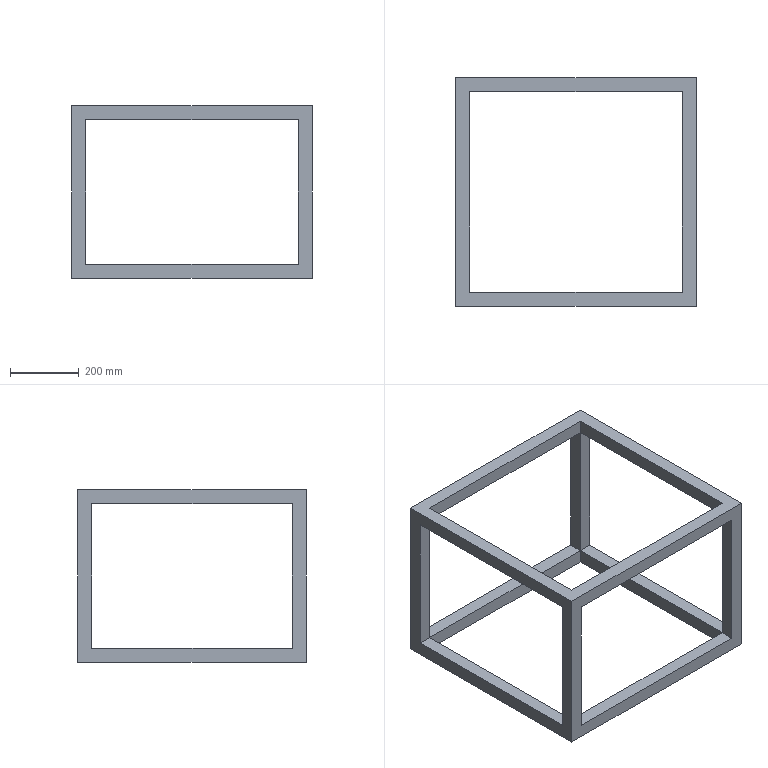Part | STEP file | Small table plate frame | 1 solid | 30 faces | box 700 x 665 x 501.75 mm | volume 10923200 mm3 | plane 30